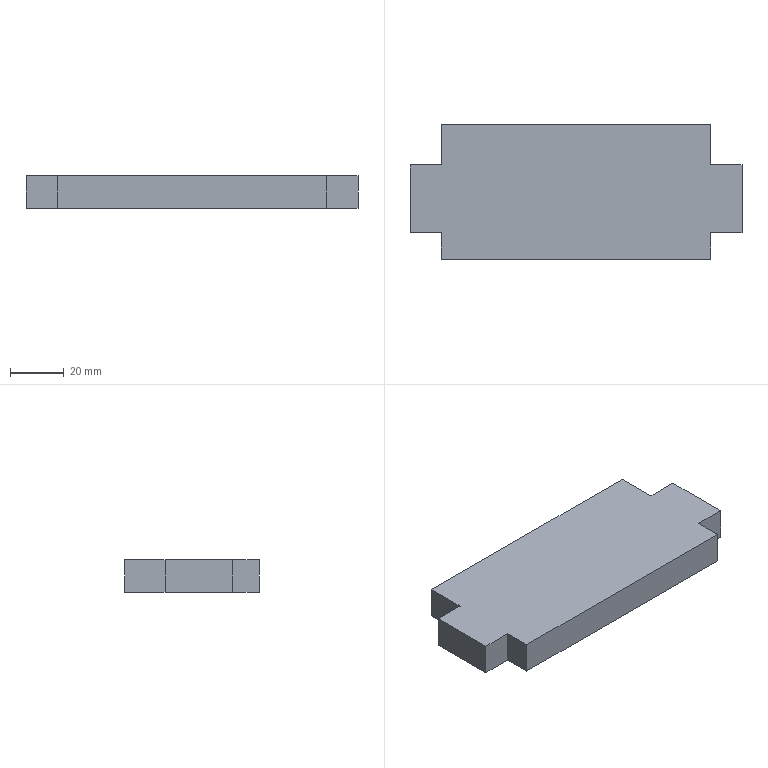Part | SolidWorks | features FlatPattern 1, SMBaseFlange 1, SheetMetal 1 | 1 solid | 14 faces | box 123 x 50 x 12 mm | volume 66900 mm3 | plane 14
STEP:
#1=CARTESIAN_POINT('',(144.45,-62.118,0.));
#2=VERTEX_POINT('',#1);
#3=CARTESIAN_POINT('',(144.45,-77.118,0.));
#4=VERTEX_POINT('',#3);
#5=CARTESIAN_POINT('',(144.45,-62.118,0.));
#6=DIRECTION('',(0.,-1.,0.));
#7=VECTOR('',#6,1000.);
#8=LINE('',#5,#7);
#9=EDGE_CURVE('',#2,#4,#8,.T.);
#10=ORIENTED_EDGE('',*,*,#9,.F.);
#11=CARTESIAN_POINT('',(144.45,-62.118,-12.));
#12=VERTEX_POINT('',#11);
#13=CARTESIAN_POINT('',(144.45,-62.118,-12.));
#14=DIRECTION('',(0.,0.,1.));
#15=VECTOR('',#14,1000.);
#16=LINE('',#13,#15);
#17=EDGE_CURVE('',#12,#2,#16,.T.);
#18=ORIENTED_EDGE('',*,*,#17,.F.);
#19=CARTESIAN_POINT('',(144.45,-77.118,-12.));
#20=VERTEX_POINT('',#19);
#21=CARTESIAN_POINT('',(144.45,-62.118,-12.));
#22=DIRECTION('',(0.,-1.,0.));
#23=VECTOR('',#22,1000.);
#24=LINE('',#21,#23);
#25=EDGE_CURVE('',#12,#20,#24,.T.);
#26=ORIENTED_EDGE('',*,*,#25,.T.);
#27=CARTESIAN_POINT('',(144.45,-77.118,-12.));
#28=DIRECTION('',(0.,0.,1.));
#29=VECTOR('',#28,1000.);
#30=LINE('',#27,#29);
#31=EDGE_CURVE('',#20,#4,#30,.T.);
#32=ORIENTED_EDGE('',*,*,#31,.T.);
#33=EDGE_LOOP('',(#10,#18,#26,#32));
#34=FACE_OUTER_BOUND('',#33,.T.);
#35=CARTESIAN_POINT('',(144.45,-62.118,-12.));
#36=DIRECTION('',(-1.,0.,0.));
#37=DIRECTION('',(0.,0.,1.));
#38=AXIS2_PLACEMENT_3D('',#35,#36,#37);
#39=PLANE('',#38);
#40=ADVANCED_FACE('',(#34),#39,.T.);
#41=CARTESIAN_POINT('',(244.45,-62.118,0.));
#42=VERTEX_POINT('',#41);
#43=CARTESIAN_POINT('',(144.45,-62.118,0.));
#44=DIRECTION('',(-1.,0.,0.));
#45=VECTOR('',#44,1000.);
#46=LINE('',#43,#45);
#47=EDGE_CURVE('',#42,#2,#46,.T.);
#48=ORIENTED_EDGE('',*,*,#47,.F.);
#49=CARTESIAN_POINT('',(244.45,-62.118,-12.));
#50=VERTEX_POINT('',#49);
#51=CARTESIAN_POINT('',(244.45,-62.118,-12.));
#52=DIRECTION('',(0.,0.,1.));
#53=VECTOR('',#52,1000.);
#54=LINE('',#51,#53);
#55=EDGE_CURVE('',#50,#42,#54,.T.);
#56=ORIENTED_EDGE('',*,*,#55,.F.);
#57=CARTESIAN_POINT('',(144.45,-62.118,-12.));
#58=DIRECTION('',(-1.,0.,0.));
#59=VECTOR('',#58,1000.);
#60=LINE('',#57,#59);
#61=EDGE_CURVE('',#50,#12,#60,.T.);
#62=ORIENTED_EDGE('',*,*,#61,.T.);
#63=ORIENTED_EDGE('',*,*,#17,.T.);
#64=EDGE_LOOP('',(#48,#56,#62,#63));
#65=FACE_OUTER_BOUND('',#64,.T.);
#66=CARTESIAN_POINT('',(144.45,-62.118,-12.));
#67=DIRECTION('',(0.,1.,0.));
#68=DIRECTION('',(0.,0.,1.));
#69=AXIS2_PLACEMENT_3D('',#66,#67,#68);
#70=PLANE('',#69);
#71=ADVANCED_FACE('',(#65),#70,.T.);
#72=CARTESIAN_POINT('',(244.45,-77.118,0.));
#73=VERTEX_POINT('',#72);
#74=CARTESIAN_POINT('',(244.45,-62.118,0.));
#75=DIRECTION('',(0.,1.,0.));
#76=VECTOR('',#75,1000.);
#77=LINE('',#74,#76);
#78=EDGE_CURVE('',#73,#42,#77,.T.);
#79=ORIENTED_EDGE('',*,*,#78,.F.);
#80=CARTESIAN_POINT('',(244.45,-77.118,-12.));
#81=VERTEX_POINT('',#80);
#82=CARTESIAN_POINT('',(244.45,-77.118,-12.));
#83=DIRECTION('',(0.,0.,1.));
#84=VECTOR('',#83,1000.);
#85=LINE('',#82,#84);
#86=EDGE_CURVE('',#81,#73,#85,.T.);
#87=ORIENTED_EDGE('',*,*,#86,.F.);
#88=CARTESIAN_POINT('',(244.45,-62.118,-12.));
#89=DIRECTION('',(0.,1.,0.));
#90=VECTOR('',#89,1000.);
#91=LINE('',#88,#90);
#92=EDGE_CURVE('',#81,#50,#91,.T.);
#93=ORIENTED_EDGE('',*,*,#92,.T.);
#94=ORIENTED_EDGE('',*,*,#55,.T.);
#95=EDGE_LOOP('',(#79,#87,#93,#94));
#96=FACE_OUTER_BOUND('',#95,.T.);
#97=CARTESIAN_POINT('',(244.45,-62.118,-12.));
#98=DIRECTION('',(1.,0.,0.));
#99=DIRECTION('',(0.,0.,-1.));
#100=AXIS2_PLACEMENT_3D('',#97,#98,#99);
#101=PLANE('',#100);
#102=ADVANCED_FACE('',(#96),#101,.T.);
#103=CARTESIAN_POINT('',(255.95,-77.118,0.));
#104=VERTEX_POINT('',#103);
#105=CARTESIAN_POINT('',(244.45,-77.118,0.));
#106=DIRECTION('',(-1.,0.,0.));
#107=VECTOR('',#106,1000.);
#108=LINE('',#105,#107);
#109=EDGE_CURVE('',#104,#73,#108,.T.);
#110=ORIENTED_EDGE('',*,*,#109,.F.);
#111=CARTESIAN_POINT('',(255.95,-77.118,-12.));
#112=VERTEX_POINT('',#111);
#113=CARTESIAN_POINT('',(255.95,-77.118,-12.));
#114=DIRECTION('',(0.,0.,1.));
#115=VECTOR('',#114,1000.);
#116=LINE('',#113,#115);
#117=EDGE_CURVE('',#112,#104,#116,.T.);
#118=ORIENTED_EDGE('',*,*,#117,.F.);
#119=CARTESIAN_POINT('',(244.45,-77.118,-12.));
#120=DIRECTION('',(-1.,0.,0.));
#121=VECTOR('',#120,1000.);
#122=LINE('',#119,#121);
#123=EDGE_CURVE('',#112,#81,#122,.T.);
#124=ORIENTED_EDGE('',*,*,#123,.T.);
#125=ORIENTED_EDGE('',*,*,#86,.T.);
#126=EDGE_LOOP('',(#110,#118,#124,#125));
#127=FACE_OUTER_BOUND('',#126,.T.);
#128=CARTESIAN_POINT('',(244.45,-77.118,-12.));
#129=DIRECTION('',(0.,1.,0.));
#130=DIRECTION('',(0.,0.,1.));
#131=AXIS2_PLACEMENT_3D('',#128,#129,#130);
#132=PLANE('',#131);
#133=ADVANCED_FACE('',(#127),#132,.T.);
#134=CARTESIAN_POINT('',(255.95,-102.118,0.));
#135=VERTEX_POINT('',#134);
#136=CARTESIAN_POINT('',(255.95,-77.118,0.));
#137=DIRECTION('',(0.,1.,0.));
#138=VECTOR('',#137,1000.);
#139=LINE('',#136,#138);
#140=EDGE_CURVE('',#135,#104,#139,.T.);
#141=ORIENTED_EDGE('',*,*,#140,.F.);
#142=CARTESIAN_POINT('',(255.95,-102.118,-12.));
#143=VERTEX_POINT('',#142);
#144=CARTESIAN_POINT('',(255.95,-102.118,-12.));
#145=DIRECTION('',(0.,0.,1.));
#146=VECTOR('',#145,1000.);
#147=LINE('',#144,#146);
#148=EDGE_CURVE('',#143,#135,#147,.T.);
#149=ORIENTED_EDGE('',*,*,#148,.F.);
#150=CARTESIAN_POINT('',(255.95,-77.118,-12.));
#151=DIRECTION('',(0.,1.,0.));
#152=VECTOR('',#151,1000.);
#153=LINE('',#150,#152);
#154=EDGE_CURVE('',#143,#112,#153,.T.);
#155=ORIENTED_EDGE('',*,*,#154,.T.);
#156=ORIENTED_EDGE('',*,*,#117,.T.);
#157=EDGE_LOOP('',(#141,#149,#155,#156));
#158=FACE_OUTER_BOUND('',#157,.T.);
#159=CARTESIAN_POINT('',(255.95,-77.118,-12.));
#160=DIRECTION('',(1.,0.,0.));
#161=DIRECTION('',(0.,0.,-1.));
#162=AXIS2_PLACEMENT_3D('',#159,#160,#161);
#163=PLANE('',#162);
#164=ADVANCED_FACE('',(#158),#163,.T.);
#165=CARTESIAN_POINT('',(244.45,-102.118,0.));
#166=VERTEX_POINT('',#165);
#167=CARTESIAN_POINT('',(255.95,-102.118,0.));
#168=DIRECTION('',(1.,0.,0.));
#169=VECTOR('',#168,1000.);
#170=LINE('',#167,#169);
#171=EDGE_CURVE('',#166,#135,#170,.T.);
#172=ORIENTED_EDGE('',*,*,#171,.F.);
#173=CARTESIAN_POINT('',(244.45,-102.118,-12.));
#174=VERTEX_POINT('',#173);
#175=CARTESIAN_POINT('',(244.45,-102.118,-12.));
#176=DIRECTION('',(0.,0.,1.));
#177=VECTOR('',#176,1000.);
#178=LINE('',#175,#177);
#179=EDGE_CURVE('',#174,#166,#178,.T.);
#180=ORIENTED_EDGE('',*,*,#179,.F.);
#181=CARTESIAN_POINT('',(255.95,-102.118,-12.));
#182=DIRECTION('',(1.,0.,0.));
#183=VECTOR('',#182,1000.);
#184=LINE('',#181,#183);
#185=EDGE_CURVE('',#174,#143,#184,.T.);
#186=ORIENTED_EDGE('',*,*,#185,.T.);
#187=ORIENTED_EDGE('',*,*,#148,.T.);
#188=EDGE_LOOP('',(#172,#180,#186,#187));
#189=FACE_OUTER_BOUND('',#188,.T.);
#190=CARTESIAN_POINT('',(255.95,-102.118,-12.));
#191=DIRECTION('',(0.,-1.,0.));
#192=DIRECTION('',(0.,0.,-1.));
#193=AXIS2_PLACEMENT_3D('',#190,#191,#192);
#194=PLANE('',#193);
#195=ADVANCED_FACE('',(#189),#194,.T.);
#196=CARTESIAN_POINT('',(244.45,-112.118,0.));
#197=VERTEX_POINT('',#196);
#198=CARTESIAN_POINT('',(244.45,-102.118,0.));
#199=DIRECTION('',(0.,1.,0.));
#200=VECTOR('',#199,1000.);
#201=LINE('',#198,#200);
#202=EDGE_CURVE('',#197,#166,#201,.T.);
#203=ORIENTED_EDGE('',*,*,#202,.F.);
#204=CARTESIAN_POINT('',(244.45,-112.118,-12.));
#205=VERTEX_POINT('',#204);
#206=CARTESIAN_POINT('',(244.45,-112.118,-12.));
#207=DIRECTION('',(0.,0.,1.));
#208=VECTOR('',#207,1000.);
#209=LINE('',#206,#208);
#210=EDGE_CURVE('',#205,#197,#209,.T.);
#211=ORIENTED_EDGE('',*,*,#210,.F.);
#212=CARTESIAN_POINT('',(244.45,-102.118,-12.));
#213=DIRECTION('',(0.,1.,0.));
#214=VECTOR('',#213,1000.);
#215=LINE('',#212,#214);
#216=EDGE_CURVE('',#205,#174,#215,.T.);
#217=ORIENTED_EDGE('',*,*,#216,.T.);
#218=ORIENTED_EDGE('',*,*,#179,.T.);
#219=EDGE_LOOP('',(#203,#211,#217,#218));
#220=FACE_OUTER_BOUND('',#219,.T.);
#221=CARTESIAN_POINT('',(244.45,-102.118,-12.));
#222=DIRECTION('',(1.,0.,0.));
#223=DIRECTION('',(0.,0.,-1.));
#224=AXIS2_PLACEMENT_3D('',#221,#222,#223);
#225=PLANE('',#224);
#226=ADVANCED_FACE('',(#220),#225,.T.);
#227=CARTESIAN_POINT('',(144.45,-112.118,0.));
#228=VERTEX_POINT('',#227);
#229=CARTESIAN_POINT('',(144.45,-112.118,0.));
#230=DIRECTION('',(1.,0.,0.));
#231=VECTOR('',#230,1000.);
#232=LINE('',#229,#231);
#233=EDGE_CURVE('',#228,#197,#232,.T.);
#234=ORIENTED_EDGE('',*,*,#233,.F.);
#235=CARTESIAN_POINT('',(144.45,-112.118,-12.));
#236=VERTEX_POINT('',#235);
#237=CARTESIAN_POINT('',(144.45,-112.118,-12.));
#238=DIRECTION('',(0.,0.,1.));
#239=VECTOR('',#238,1000.);
#240=LINE('',#237,#239);
#241=EDGE_CURVE('',#236,#228,#240,.T.);
#242=ORIENTED_EDGE('',*,*,#241,.F.);
#243=CARTESIAN_POINT('',(144.45,-112.118,-12.));
#244=DIRECTION('',(1.,0.,0.));
#245=VECTOR('',#244,1000.);
#246=LINE('',#243,#245);
#247=EDGE_CURVE('',#236,#205,#246,.T.);
#248=ORIENTED_EDGE('',*,*,#247,.T.);
#249=ORIENTED_EDGE('',*,*,#210,.T.);
#250=EDGE_LOOP('',(#234,#242,#248,#249));
#251=FACE_OUTER_BOUND('',#250,.T.);
#252=CARTESIAN_POINT('',(144.45,-112.118,-12.));
#253=DIRECTION('',(0.,-1.,0.));
#254=DIRECTION('',(0.,0.,-1.));
#255=AXIS2_PLACEMENT_3D('',#252,#253,#254);
#256=PLANE('',#255);
#257=ADVANCED_FACE('',(#251),#256,.T.);
#258=CARTESIAN_POINT('',(144.45,-102.118,0.));
#259=VERTEX_POINT('',#258);
#260=CARTESIAN_POINT('',(144.45,-102.118,0.));
#261=DIRECTION('',(0.,-1.,0.));
#262=VECTOR('',#261,1000.);
#263=LINE('',#260,#262);
#264=EDGE_CURVE('',#259,#228,#263,.T.);
#265=ORIENTED_EDGE('',*,*,#264,.F.);
#266=CARTESIAN_POINT('',(144.45,-102.118,-12.));
#267=VERTEX_POINT('',#266);
#268=CARTESIAN_POINT('',(144.45,-102.118,-12.));
#269=DIRECTION('',(0.,0.,1.));
#270=VECTOR('',#269,1000.);
#271=LINE('',#268,#270);
#272=EDGE_CURVE('',#267,#259,#271,.T.);
#273=ORIENTED_EDGE('',*,*,#272,.F.);
#274=CARTESIAN_POINT('',(144.45,-102.118,-12.));
#275=DIRECTION('',(0.,-1.,0.));
#276=VECTOR('',#275,1000.);
#277=LINE('',#274,#276);
#278=EDGE_CURVE('',#267,#236,#277,.T.);
#279=ORIENTED_EDGE('',*,*,#278,.T.);
#280=ORIENTED_EDGE('',*,*,#241,.T.);
#281=EDGE_LOOP('',(#265,#273,#279,#280));
#282=FACE_OUTER_BOUND('',#281,.T.);
#283=CARTESIAN_POINT('',(144.45,-102.118,-12.));
#284=DIRECTION('',(-1.,0.,0.));
#285=DIRECTION('',(0.,0.,1.));
#286=AXIS2_PLACEMENT_3D('',#283,#284,#285);
#287=PLANE('',#286);
#288=ADVANCED_FACE('',(#282),#287,.T.);
#289=CARTESIAN_POINT('',(132.95,-102.118,0.));
#290=VERTEX_POINT('',#289);
#291=CARTESIAN_POINT('',(132.95,-102.118,0.));
#292=DIRECTION('',(1.,0.,0.));
#293=VECTOR('',#292,1000.);
#294=LINE('',#291,#293);
#295=EDGE_CURVE('',#290,#259,#294,.T.);
#296=ORIENTED_EDGE('',*,*,#295,.F.);
#297=CARTESIAN_POINT('',(132.95,-102.118,-12.));
#298=VERTEX_POINT('',#297);
#299=CARTESIAN_POINT('',(132.95,-102.118,-12.));
#300=DIRECTION('',(0.,0.,1.));
#301=VECTOR('',#300,1000.);
#302=LINE('',#299,#301);
#303=EDGE_CURVE('',#298,#290,#302,.T.);
#304=ORIENTED_EDGE('',*,*,#303,.F.);
#305=CARTESIAN_POINT('',(132.95,-102.118,-12.));
#306=DIRECTION('',(1.,0.,0.));
#307=VECTOR('',#306,1000.);
#308=LINE('',#305,#307);
#309=EDGE_CURVE('',#298,#267,#308,.T.);
#310=ORIENTED_EDGE('',*,*,#309,.T.);
#311=ORIENTED_EDGE('',*,*,#272,.T.);
#312=EDGE_LOOP('',(#296,#304,#310,#311));
#313=FACE_OUTER_BOUND('',#312,.T.);
#314=CARTESIAN_POINT('',(132.95,-102.118,-12.));
#315=DIRECTION('',(0.,-1.,0.));
#316=DIRECTION('',(0.,0.,-1.));
#317=AXIS2_PLACEMENT_3D('',#314,#315,#316);
#318=PLANE('',#317);
#319=ADVANCED_FACE('',(#313),#318,.T.);
#320=CARTESIAN_POINT('',(132.95,-77.118,0.));
#321=VERTEX_POINT('',#320);
#322=CARTESIAN_POINT('',(132.95,-77.118,0.));
#323=DIRECTION('',(0.,-1.,0.));
#324=VECTOR('',#323,1000.);
#325=LINE('',#322,#324);
#326=EDGE_CURVE('',#321,#290,#325,.T.);
#327=ORIENTED_EDGE('',*,*,#326,.F.);
#328=CARTESIAN_POINT('',(132.95,-77.118,-12.));
#329=VERTEX_POINT('',#328);
#330=CARTESIAN_POINT('',(132.95,-77.118,-12.));
#331=DIRECTION('',(0.,0.,1.));
#332=VECTOR('',#331,1000.);
#333=LINE('',#330,#332);
#334=EDGE_CURVE('',#329,#321,#333,.T.);
#335=ORIENTED_EDGE('',*,*,#334,.F.);
#336=CARTESIAN_POINT('',(132.95,-77.118,-12.));
#337=DIRECTION('',(0.,-1.,0.));
#338=VECTOR('',#337,1000.);
#339=LINE('',#336,#338);
#340=EDGE_CURVE('',#329,#298,#339,.T.);
#341=ORIENTED_EDGE('',*,*,#340,.T.);
#342=ORIENTED_EDGE('',*,*,#303,.T.);
#343=EDGE_LOOP('',(#327,#335,#341,#342));
#344=FACE_OUTER_BOUND('',#343,.T.);
#345=CARTESIAN_POINT('',(132.95,-77.118,-12.));
#346=DIRECTION('',(-1.,0.,0.));
#347=DIRECTION('',(0.,0.,1.));
#348=AXIS2_PLACEMENT_3D('',#345,#346,#347);
#349=PLANE('',#348);
#350=ADVANCED_FACE('',(#344),#349,.T.);
#351=CARTESIAN_POINT('',(144.45,-77.118,0.));
#352=DIRECTION('',(-1.,0.,0.));
#353=VECTOR('',#352,1000.);
#354=LINE('',#351,#353);
#355=EDGE_CURVE('',#4,#321,#354,.T.);
#356=ORIENTED_EDGE('',*,*,#355,.F.);
#357=ORIENTED_EDGE('',*,*,#31,.F.);
#358=CARTESIAN_POINT('',(144.45,-77.118,-12.));
#359=DIRECTION('',(-1.,0.,0.));
#360=VECTOR('',#359,1000.);
#361=LINE('',#358,#360);
#362=EDGE_CURVE('',#20,#329,#361,.T.);
#363=ORIENTED_EDGE('',*,*,#362,.T.);
#364=ORIENTED_EDGE('',*,*,#334,.T.);
#365=EDGE_LOOP('',(#356,#357,#363,#364));
#366=FACE_OUTER_BOUND('',#365,.T.);
#367=CARTESIAN_POINT('',(144.45,-77.118,-12.));
#368=DIRECTION('',(0.,1.,0.));
#369=DIRECTION('',(0.,0.,1.));
#370=AXIS2_PLACEMENT_3D('',#367,#368,#369);
#371=PLANE('',#370);
#372=ADVANCED_FACE('',(#366),#371,.T.);
#373=ORIENTED_EDGE('',*,*,#25,.F.);
#374=ORIENTED_EDGE('',*,*,#61,.F.);
#375=ORIENTED_EDGE('',*,*,#92,.F.);
#376=ORIENTED_EDGE('',*,*,#123,.F.);
#377=ORIENTED_EDGE('',*,*,#154,.F.);
#378=ORIENTED_EDGE('',*,*,#185,.F.);
#379=ORIENTED_EDGE('',*,*,#216,.F.);
#380=ORIENTED_EDGE('',*,*,#247,.F.);
#381=ORIENTED_EDGE('',*,*,#278,.F.);
#382=ORIENTED_EDGE('',*,*,#309,.F.);
#383=ORIENTED_EDGE('',*,*,#340,.F.);
#384=ORIENTED_EDGE('',*,*,#362,.F.);
#385=EDGE_LOOP('',(#373,#374,#375,#376,#377,#378,#379,#380,#381,#382,#383,#384));
#386=FACE_OUTER_BOUND('',#385,.T.);
#387=CARTESIAN_POINT('',(0.,0.,-12.));
#388=DIRECTION('',(0.,0.,-1.));
#389=DIRECTION('',(-1.,0.,0.));
#390=AXIS2_PLACEMENT_3D('',#387,#388,#389);
#391=PLANE('',#390);
#392=ADVANCED_FACE('',(#386),#391,.T.);
#393=ORIENTED_EDGE('',*,*,#9,.T.);
#394=ORIENTED_EDGE('',*,*,#355,.T.);
#395=ORIENTED_EDGE('',*,*,#326,.T.);
#396=ORIENTED_EDGE('',*,*,#295,.T.);
#397=ORIENTED_EDGE('',*,*,#264,.T.);
#398=ORIENTED_EDGE('',*,*,#233,.T.);
#399=ORIENTED_EDGE('',*,*,#202,.T.);
#400=ORIENTED_EDGE('',*,*,#171,.T.);
#401=ORIENTED_EDGE('',*,*,#140,.T.);
#402=ORIENTED_EDGE('',*,*,#109,.T.);
#403=ORIENTED_EDGE('',*,*,#78,.T.);
#404=ORIENTED_EDGE('',*,*,#47,.T.);
#405=EDGE_LOOP('',(#393,#394,#395,#396,#397,#398,#399,#400,#401,#402,#403,#404));
#406=FACE_OUTER_BOUND('',#405,.T.);
#407=CARTESIAN_POINT('',(0.,0.,0.));
#408=DIRECTION('',(0.,0.,-1.));
#409=DIRECTION('',(-1.,0.,0.));
#410=AXIS2_PLACEMENT_3D('',#407,#408,#409);
#411=PLANE('',#410);
#412=ADVANCED_FACE('',(#406),#411,.F.);
#413=CLOSED_SHELL('',(#40,#71,#102,#133,#164,#195,#226,#257,#288,#319,#350,#372,#392,#412));
#414=MANIFOLD_SOLID_BREP('',#413);
#415=CARTESIAN_POINT('',(0.,0.,0.));
#416=DIRECTION('',(0.,0.,1.));
#417=DIRECTION('',(1.,0.,0.));
#418=AXIS2_PLACEMENT_3D('',#415,#416,#417);
#419=(LENGTH_UNIT()NAMED_UNIT(*)SI_UNIT(.MILLI.,.METRE.));
#420=UNCERTAINTY_MEASURE_WITH_UNIT(LENGTH_MEASURE(0.00001),#419,'','');
#421=(NAMED_UNIT(*)PLANE_ANGLE_UNIT()SI_UNIT($,.RADIAN.));
#422=(NAMED_UNIT(*)SI_UNIT($,.STERADIAN.)SOLID_ANGLE_UNIT());
#423=(GEOMETRIC_REPRESENTATION_CONTEXT(3)GLOBAL_UNCERTAINTY_ASSIGNED_CONTEXT((#420))GLOBAL_UNIT_ASSIGNED_CONTEXT((#419,#421,#422))REPRESENTATION_CONTEXT('',''));
#424=ADVANCED_BREP_SHAPE_REPRESENTATION('',(#414,#418),#423);